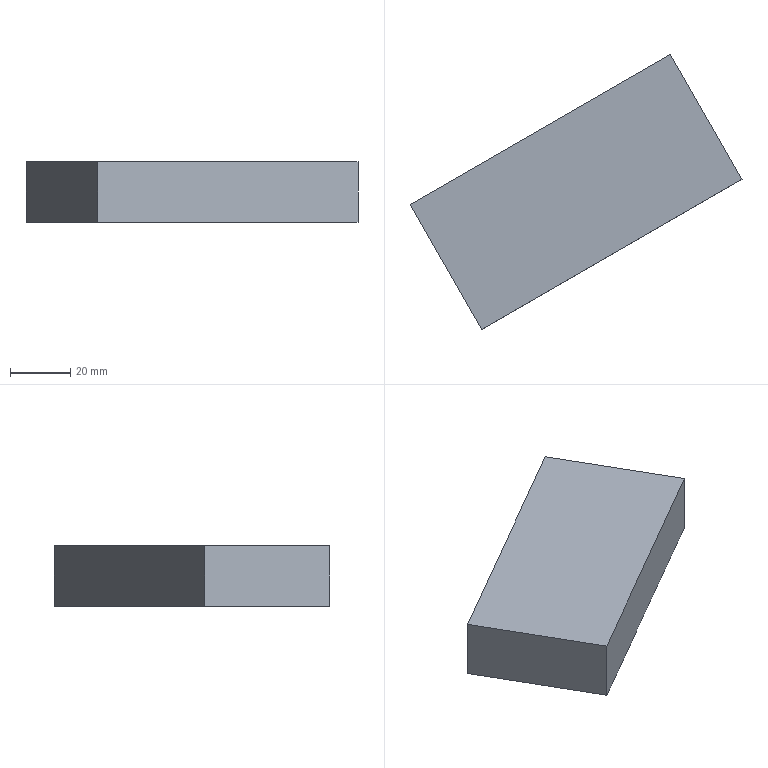Part | NX | features solid 2 | 1 solid | 6 faces | box 110.479 x 91.641 x 20 mm | volume 96000 mm3 | plane 6
STEP:
#1=CARTESIAN_POINT('',(-901.573,19.118,-210.));
#2=VERTEX_POINT('',#1);
#3=CARTESIAN_POINT('',(-988.176,-30.882,-210.));
#4=VERTEX_POINT('',#3);
#5=CARTESIAN_POINT('',(-910.11,14.189,-210.));
#6=DIRECTION('',(-0.866,-0.5,0.));
#7=VECTOR('',#6,1000.);
#8=LINE('',#5,#7);
#9=EDGE_CURVE('',#2,#4,#8,.T.);
#10=ORIENTED_EDGE('',*,*,#9,.T.);
#11=CARTESIAN_POINT('',(-988.176,-30.882,-230.));
#12=VERTEX_POINT('',#11);
#13=CARTESIAN_POINT('',(-988.176,-30.882,-230.));
#14=DIRECTION('',(0.,0.,1.));
#15=VECTOR('',#14,1000.);
#16=LINE('',#13,#15);
#17=EDGE_CURVE('',#12,#4,#16,.T.);
#18=ORIENTED_EDGE('',*,*,#17,.F.);
#19=CARTESIAN_POINT('',(-901.573,19.118,-230.));
#20=VERTEX_POINT('',#19);
#21=CARTESIAN_POINT('',(-910.11,14.189,-230.));
#22=DIRECTION('',(-0.866,-0.5,0.));
#23=VECTOR('',#22,1000.);
#24=LINE('',#21,#23);
#25=EDGE_CURVE('',#20,#12,#24,.T.);
#26=ORIENTED_EDGE('',*,*,#25,.F.);
#27=CARTESIAN_POINT('',(-901.573,19.118,-200.));
#28=DIRECTION('',(0.,0.,1.));
#29=VECTOR('',#28,1000.);
#30=LINE('',#27,#29);
#31=EDGE_CURVE('',#20,#2,#30,.T.);
#32=ORIENTED_EDGE('',*,*,#31,.T.);
#33=EDGE_LOOP('',(#10,#18,#26,#32));
#34=FACE_BOUND('',#33,.T.);
#35=CARTESIAN_POINT('',(-910.11,14.189,-200.));
#36=DIRECTION('',(0.5,-0.866,0.));
#37=DIRECTION('',(0.866,0.5,0.));
#38=AXIS2_PLACEMENT_3D('',#35,#36,#37);
#39=PLANE('',#38);
#40=ADVANCED_FACE('',(#34),#39,.T.);
#41=CARTESIAN_POINT('',(-925.45,60.759,-210.));
#42=VERTEX_POINT('',#41);
#43=CARTESIAN_POINT('',(-896.644,10.522,-210.));
#44=DIRECTION('',(0.4974,-0.8675,0.));
#45=VECTOR('',#44,1000.);
#46=LINE('',#43,#45);
#47=EDGE_CURVE('',#42,#2,#46,.T.);
#48=ORIENTED_EDGE('',*,*,#47,.T.);
#49=ORIENTED_EDGE('',*,*,#31,.F.);
#50=CARTESIAN_POINT('',(-925.45,60.759,-230.));
#51=VERTEX_POINT('',#50);
#52=CARTESIAN_POINT('',(-896.644,10.522,-230.));
#53=DIRECTION('',(0.4974,-0.8675,0.));
#54=VECTOR('',#53,1000.);
#55=LINE('',#52,#54);
#56=EDGE_CURVE('',#51,#20,#55,.T.);
#57=ORIENTED_EDGE('',*,*,#56,.F.);
#58=CARTESIAN_POINT('',(-925.45,60.759,-230.));
#59=DIRECTION('',(0.,0.,1.));
#60=VECTOR('',#59,1000.);
#61=LINE('',#58,#60);
#62=EDGE_CURVE('',#51,#42,#61,.T.);
#63=ORIENTED_EDGE('',*,*,#62,.T.);
#64=EDGE_LOOP('',(#48,#49,#57,#63));
#65=FACE_BOUND('',#64,.T.);
#66=CARTESIAN_POINT('',(-896.644,10.522,-230.));
#67=DIRECTION('',(0.8675,0.4974,0.));
#68=DIRECTION('',(0.4974,-0.8675,0.));
#69=AXIS2_PLACEMENT_3D('',#66,#67,#68);
#70=PLANE('',#69);
#71=ADVANCED_FACE('',(#65),#70,.T.);
#72=CARTESIAN_POINT('',(-1012.052,10.759,-210.));
#73=VERTEX_POINT('',#72);
#74=CARTESIAN_POINT('',(-934.11,55.758,-210.));
#75=DIRECTION('',(0.866,0.5,0.));
#76=VECTOR('',#75,1000.);
#77=LINE('',#74,#76);
#78=EDGE_CURVE('',#73,#42,#77,.T.);
#79=ORIENTED_EDGE('',*,*,#78,.T.);
#80=ORIENTED_EDGE('',*,*,#62,.F.);
#81=CARTESIAN_POINT('',(-1012.052,10.759,-230.));
#82=VERTEX_POINT('',#81);
#83=CARTESIAN_POINT('',(-934.11,55.758,-230.));
#84=DIRECTION('',(0.866,0.5,0.));
#85=VECTOR('',#84,1000.);
#86=LINE('',#83,#85);
#87=EDGE_CURVE('',#82,#51,#86,.T.);
#88=ORIENTED_EDGE('',*,*,#87,.F.);
#89=CARTESIAN_POINT('',(-1012.052,10.759,-230.));
#90=DIRECTION('',(0.,0.,1.));
#91=VECTOR('',#90,1000.);
#92=LINE('',#89,#91);
#93=EDGE_CURVE('',#82,#73,#92,.T.);
#94=ORIENTED_EDGE('',*,*,#93,.T.);
#95=EDGE_LOOP('',(#79,#80,#88,#94));
#96=FACE_BOUND('',#95,.T.);
#97=CARTESIAN_POINT('',(-934.11,55.758,-230.));
#98=DIRECTION('',(-0.5,0.866,0.));
#99=DIRECTION('',(0.866,0.5,0.));
#100=AXIS2_PLACEMENT_3D('',#97,#98,#99);
#101=PLANE('',#100);
#102=ADVANCED_FACE('',(#96),#101,.T.);
#103=CARTESIAN_POINT('',(-983.395,-39.22,-210.));
#104=DIRECTION('',(-0.4974,0.8675,0.));
#105=VECTOR('',#104,1000.);
#106=LINE('',#103,#105);
#107=EDGE_CURVE('',#4,#73,#106,.T.);
#108=ORIENTED_EDGE('',*,*,#107,.T.);
#109=ORIENTED_EDGE('',*,*,#93,.F.);
#110=CARTESIAN_POINT('',(-983.395,-39.22,-230.));
#111=DIRECTION('',(-0.4974,0.8675,0.));
#112=VECTOR('',#111,1000.);
#113=LINE('',#110,#112);
#114=EDGE_CURVE('',#12,#82,#113,.T.);
#115=ORIENTED_EDGE('',*,*,#114,.F.);
#116=ORIENTED_EDGE('',*,*,#17,.T.);
#117=EDGE_LOOP('',(#108,#109,#115,#116));
#118=FACE_BOUND('',#117,.T.);
#119=CARTESIAN_POINT('',(-983.395,-39.22,-230.));
#120=DIRECTION('',(-0.8675,-0.4974,0.));
#121=DIRECTION('',(-0.4974,0.8675,0.));
#122=AXIS2_PLACEMENT_3D('',#119,#120,#121);
#123=PLANE('',#122);
#124=ADVANCED_FACE('',(#118),#123,.T.);
#125=ORIENTED_EDGE('',*,*,#25,.T.);
#126=ORIENTED_EDGE('',*,*,#114,.T.);
#127=ORIENTED_EDGE('',*,*,#87,.T.);
#128=ORIENTED_EDGE('',*,*,#56,.T.);
#129=EDGE_LOOP('',(#125,#126,#127,#128));
#130=FACE_BOUND('',#129,.T.);
#131=CARTESIAN_POINT('',(-905.171,5.633,-230.));
#132=DIRECTION('',(0.,0.,1.));
#133=DIRECTION('',(-0.8675,-0.4974,0.));
#134=AXIS2_PLACEMENT_3D('',#131,#132,#133);
#135=PLANE('',#134);
#136=ADVANCED_FACE('',(#130),#135,.F.);
#137=ORIENTED_EDGE('',*,*,#9,.F.);
#138=ORIENTED_EDGE('',*,*,#47,.F.);
#139=ORIENTED_EDGE('',*,*,#78,.F.);
#140=ORIENTED_EDGE('',*,*,#107,.F.);
#141=EDGE_LOOP('',(#137,#138,#139,#140));
#142=FACE_BOUND('',#141,.T.);
#143=CARTESIAN_POINT('',(-905.171,5.633,-210.));
#144=DIRECTION('',(0.,0.,1.));
#145=DIRECTION('',(-0.8675,-0.4974,0.));
#146=AXIS2_PLACEMENT_3D('',#143,#144,#145);
#147=PLANE('',#146);
#148=ADVANCED_FACE('',(#142),#147,.T.);
#149=CLOSED_SHELL('',(#40,#71,#102,#124,#136,#148));
#150=MANIFOLD_SOLID_BREP('',#149);
#151=(LENGTH_UNIT()NAMED_UNIT(*)SI_UNIT(.MILLI.,.METRE.));
#152=UNCERTAINTY_MEASURE_WITH_UNIT(LENGTH_MEASURE(0.00001),#151,'','');
#153=(NAMED_UNIT(*)PLANE_ANGLE_UNIT()SI_UNIT($,.RADIAN.));
#154=(NAMED_UNIT(*)SI_UNIT($,.STERADIAN.)SOLID_ANGLE_UNIT());
#155=(GEOMETRIC_REPRESENTATION_CONTEXT(3)GLOBAL_UNCERTAINTY_ASSIGNED_CONTEXT((#152))GLOBAL_UNIT_ASSIGNED_CONTEXT((#151,#153,#154))REPRESENTATION_CONTEXT('',''));
#156=ADVANCED_BREP_SHAPE_REPRESENTATION('',(#150),#155);